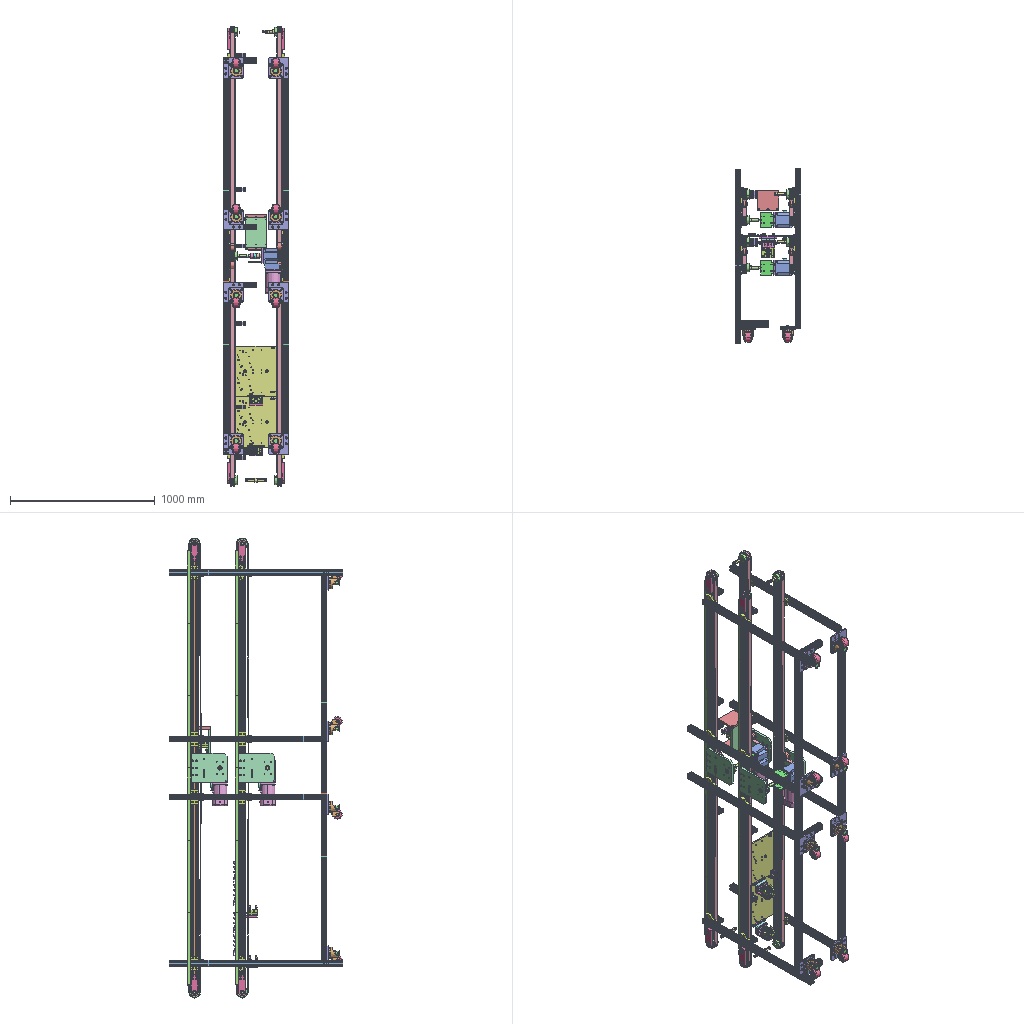Assembly | STEP file | 55 different items | 353 placed | box 456 x 1200 x 3179 mm
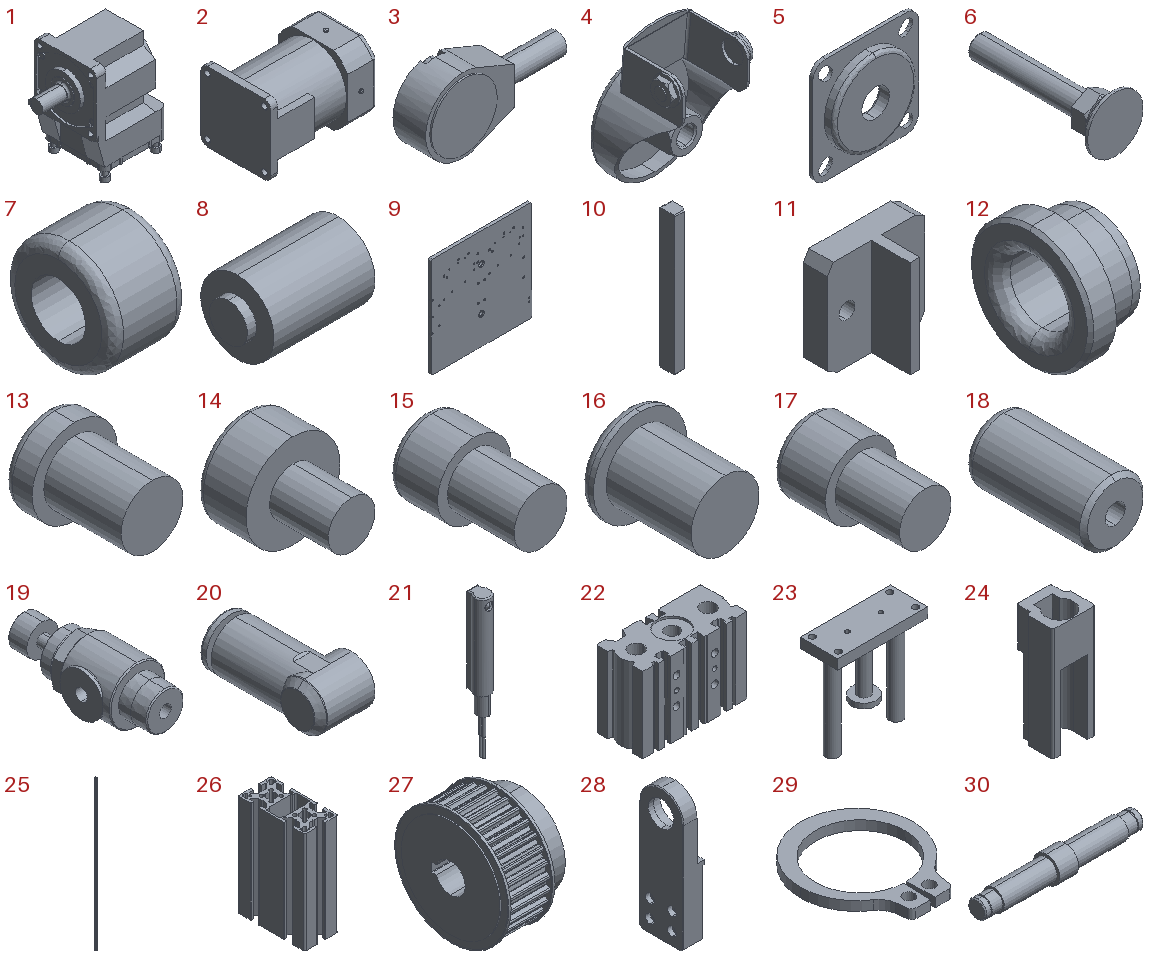Parts list (item | name | quantity | parent item | size | volume):
1 | - | x2 | in OM-BHI62E-5RA-CC05AC33P-EPCR1201-2_BHI62F_5RA_BH6G2_5RA05_, OM-BHI62E-5RA-CC05AC33P-EPCR1201-2_BHI62F_5RA_BH6G2_5RA05_-1 | 166 x 104 x 172.5 mm | 1495766 mm3
2 | OM-BHI62E-5RA-CC05AC33P-EPCR1201-2_200W_A_Motor-1 | x2 | in OM-BHI62E-5RA-CC05AC33P-EPCR1201-2_BHI62F_5RA_BH6G2_5RA05_, OM-BHI62E-5RA-CC05AC33P-EPCR1201-2_BHI62F_5RA_BH6G2_5RA05_-1 | 160 x 107.8 x 107.8 mm | 1356230 mm3
3 | OM-BHI62E-5RA-CC05AC33P-EPCR1201-2_Cable-1 | x2 | in OM-BHI62E-5RA-CC05AC33P-EPCR1201-2_BHI62F_5RA_BH6G2_5RA05_, OM-BHI62E-5RA-CC05AC33P-EPCR1201-2_BHI62F_5RA_BH6G2_5RA05_-1 | 53.5 x 14 x 27 mm | 9959 mm3
4 | CMA-2 | x8 | in CMAS65-F, CMAS65-F-1, CMAS65-F-2, CMAS65-F-3, CMAS65-F-4, CMAS65-F-5, CMAS65-F-6, CMAS65-F-7 | 80 x 61.3 x 107.359 mm | 51155 mm3
5 | CMA-1 | x8 | in CMAS65-F, CMAS65-F-1, CMAS65-F-2, CMAS65-F-3, CMAS65-F-4, CMAS65-F-5, CMAS65-F-6, CMAS65-F-7 | 102 x 12.8 x 102 mm | 66491 mm3
6 | CMA-5 | x8 | in CMAS65-F, CMAS65-F-1, CMAS65-F-2, CMAS65-F-3, CMAS65-F-4, CMAS65-F-5, CMAS65-F-6, CMAS65-F-7 | 40 x 98.8 x 40 mm | 27608 mm3
7 | CMA-4 | x8 | in CMAS65-F, CMAS65-F-1, CMAS65-F-2, CMAS65-F-3, CMAS65-F-4, CMAS65-F-5, CMAS65-F-6, CMAS65-F-7 | 45 x 65 x 65 mm | 108456 mm3
8 | CMA-3 | x8 | in CMAS65-F, CMAS65-F-1, CMAS65-F-2, CMAS65-F-3, CMAS65-F-4, CMAS65-F-5, CMAS65-F-6, CMAS65-F-7 | 53 x 32.5 x 32.5 mm | 39125 mm3
9 | PALL-001 | x2 | in PALL-01-ASSY, PALL-01-ASSY-1 | 350 x 10 x 348.5 mm | 1203530 mm3
10 | PALL-002 | x2 | in PALL-01-ASSY, PALL-01-ASSY-1 | 10 x 13 x 120 mm | 15010 mm3
11 | PALL-003 | x2 | in PALL-01-ASSY, PALL-01-ASSY-1 | 20 x 13 x 20 mm | 2211 mm3
12 | JBHM10-6 | x4 | in PALL-01-ASSY, PALL-01-ASSY-1 | 10 x 19 x 19 mm | 1348 mm3
13 | PALL-004 | x4 | in PALL-01-ASSY, PALL-01-ASSY-1 | 5.5 x 6.8 x 5.5 mm | 104.707 mm3
14 | PALL-005 | x8 | in PALL-01-ASSY, PALL-01-ASSY-1 | 8 x 9.13 x 8 mm | 269.118 mm3
15 | PALL-006 | x4 | in PALL-01-ASSY, PALL-01-ASSY-1 | 5.5 x 8.65 x 5.5 mm | 148.66 mm3
16 | PALL-007 | x8 | in PALL-01-ASSY, PALL-01-ASSY-1 | 5.5 x 5.8 x 5.5 mm | 80.949 mm3
17 | PALL-008 | x4 | in PALL-01-ASSY, PALL-01-ASSY-1 | 5.5 x 9.05 x 5.5 mm | 158.164 mm3
18 | PALL-009 | x44 | in PALL-01-ASSY, PALL-01-ASSY-1 | 8 x 15 x 8 mm | 707.835 mm3
19 | MGPL25-30-M9BL-U06US_AS3054 Body(23-01-06) | x6 | in MGPL25-30-M9BL-U06US_AS3054(AS2301F-01-06S), MGPL25-30-M9BL-U06US_AS3054(AS2301F-01-06S)-1, MGPL25-30-M9BL-U06US_AS3054(AS2301F-01-06S)-2, MGPL25-30-M9BL-U06US_AS3054(AS2301F-01-06S)-1-1, MGPL25-30-M9BL-U06US_AS3054(AS2301F-01-06S)-3, MGPL25-30-M9BL-U06US_AS3054(AS2301F-01-06S)-1-2 | 14.2 x 36.1 x 14.2 mm | 3404 mm3
20 | MGPL25-30-M9BL-U06US_AS3054 Uni Arm(2-01-06) | x6 | in MGPL25-30-M9BL-U06US_AS3054(AS2301F-01-06S), MGPL25-30-M9BL-U06US_AS3054(AS2301F-01-06S)-1, MGPL25-30-M9BL-U06US_AS3054(AS2301F-01-06S)-2, MGPL25-30-M9BL-U06US_AS3054(AS2301F-01-06S)-1-1, MGPL25-30-M9BL-U06US_AS3054(AS2301F-01-06S)-3, MGPL25-30-M9BL-U06US_AS3054(AS2301F-01-06S)-1-2 | 12.7 x 28.35 x 11.6 mm | 2524 mm3
21 | MGPL25-30-M9BL-U06US_F9_M9(M9B) | x6 | in MGPL25-30-M9BL-U06US_A9+F9+M9(M9B), MGPL25-30-M9BL-U06US_A9+F9+M9(M9B)-1, MGPL25-30-M9BL-U06US_A9+F9+M9(M9B)-2, MGPL25-30-M9BL-U06US_A9+F9+M9(M9B)-1-1, MGPL25-30-M9BL-U06US_A9+F9+M9(M9B)-3, MGPL25-30-M9BL-U06US_A9+F9+M9(M9B)-1-2 | 4 x 4.61 x 37 mm | 360.585 mm3
22 | MGPL25-30-M9BL-U06US_MGPTube(25L) | x3 | in MGPL25-30-M9BL-U06US(MGPL25-30-M9BL-U06US), MGPL25-30-M9BL-U06US(MGPL25-30-M9BL-U06US)-1, MGPL25-30-M9BL-U06US(MGPL25-30-M9BL-U06US-_flexible1) | 93 x 42 x 67.5 mm | 186060 mm3
23 | MGPL25-30-M9BL-U06US_MGPRod(25L) | x3 | in MGPL25-30-M9BL-U06US(MGPL25-30-M9BL-U06US), MGPL25-30-M9BL-U06US(MGPL25-30-M9BL-U06US)-1, MGPL25-30-M9BL-U06US(MGPL25-30-M9BL-U06US-_flexible1) | 91 x 38 x 99.5 mm | 65385 mm3
24 | MGPL25-30-M9BL-U06US_BMG2-012(Default) | x6 | in MGPL25-30-M9BL-U06US(MGPL25-30-M9BL-U06US), MGPL25-30-M9BL-U06US(MGPL25-30-M9BL-U06US)-1, MGPL25-30-M9BL-U06US(MGPL25-30-M9BL-U06US-_flexible1) | 6.2 x 5.9 x 16.5 mm | 235.85 mm3
25 | HFS5-2550-3000 | x4 | - | 25 x 50.001 x 3000 mm | 1510106 mm3
26 | HFS5-2550-300 | x11 | - | 25 x 50.001 x 76 mm | 38256 mm3
27 | HTPA30S8M250-B-N20-KC90-FC77.5-TPC5 | x12 | - | 48 x 77.5 x 77.5 mm | 160610 mm3
28 | CON-001 | x8 | - | 24 x 50 x 150 mm | 124182 mm3
29 | C Type Shaft Use Retaining Ring_jis(PreviewCfg) | x14 | - | 12.101 x 14.196 x 1 mm | 49.912 mm3
30 | CON-002 | x4 | - | 150 x 25 x 25 mm | 46152 mm3
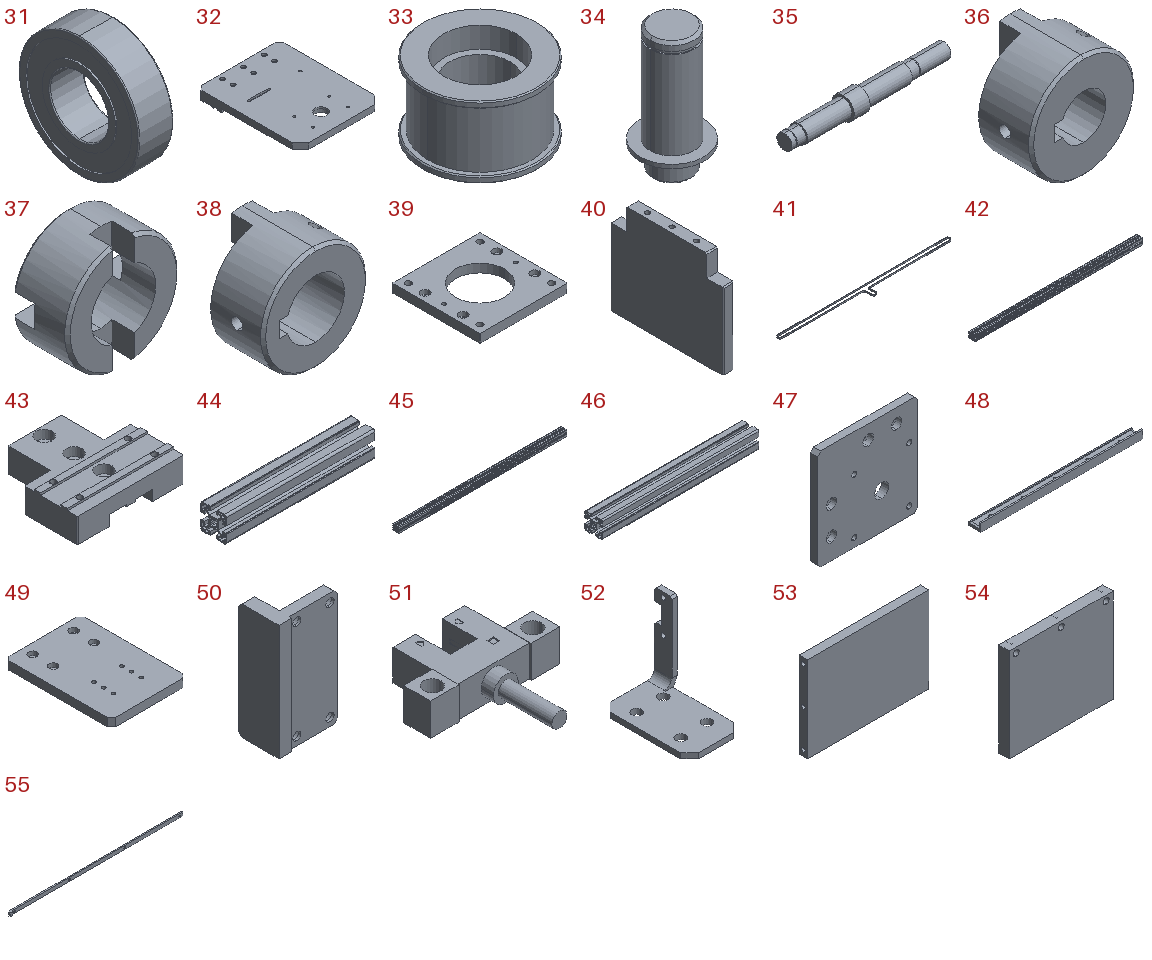31 | B6003ZZ | x25 | - | 10 x 35 x 35 mm | 7012 mm3
32 | CON-003 | x4 | - | 200 x 250 x 22 mm | 741218 mm3
33 | CON-004 | x8 | - | 55 x 55 x 34 mm | 40657 mm3
34 | CON-005 | x8 | - | 25 x 25 x 48.5 mm | 10531 mm3
35 | CON-006 | x2 | - | 180 x 25 x 25 mm | 52361 mm3
36 | CON-008 | x2 | - | 40 x 28 x 40 mm | 21406 mm3
37 | CON-009 | x2 | - | 40 x 20 x 40 mm | 14486 mm3
38 | CON-007 | x2 | - | 40 x 28 x 40 mm | 18074 mm3
39 | CON-010 | x2 | - | 104 x 104 x 10 mm | 77916 mm3
40 | CON-011 | x4 | - | 10 x 104 x 90 mm | 86051 mm3
41 | LTBR-S8M-840^ | x4 | - | 3180 x 255.872 x 25 mm | 890028 mm3
42 | AL PROFILE 4040 L 900 | x8 | - | 1050 x 40 x 40 mm | 583573 mm3
43 | CON-012 | x16 | - | 100 x 90 x 25 mm | 119624 mm3
44 | AL PROFILE 4040 L 456 | x4 | - | 233.35 x 40 x 40 mm | 129692 mm3
45 | AL PROFILE 4040 L 1110 | x4 | - | 1110 x 40 x 40 mm | 616920 mm3
46 | AL PROFILE 4040 L 360 | x2 | - | 360 x 40 x 40 mm | 200082 mm3
47 | CON-013 | x8 | - | 142 x 10 x 142 mm | 190361 mm3
48 | CON-016 | x24 | - | 500 x 37 x 24 mm | 214836 mm3
49 | CON-018 | x2 | - | 93 x 130 x 10 mm | 117582 mm3
50 | SCR-004 | x2 | - | 48 x 32 x 91 mm | 62029 mm3
51 | OMRON-EE_SX910P_R | x2 | - | 24 x 24.3 x 6 mm | 1063 mm3
52 | CON-019 | x2 | - | 33 x 50 x 47 mm | 5269 mm3
53 | CON-020 | x1 | - | 212 x 15 x 150 mm | 472548 mm3
54 | CON-021 | x2 | - | 150 x 15 x 135 mm | 298623 mm3
55 | CON-023 | x2 | - | 405 x 5 x 8 mm | 9596 mm3
Placements (level | parent | child | x y z in mm | rotation matrix by rows), first 336 of 380 lines:
1 | subassembly 2 | OM-BHI62E-5RA-CC05AC33P-EPCR1201-2_BHI62F_5RA_BH6G2_5RA05_ | 175.918 -181.25 23.458 | 0 0 -1 0 1 0 1 0 0
2 | OM-BHI62E-5RA-CC05AC33P-EPCR1201-2_BHI62F_5RA_BH6G2_5RA05_ | subassembly 3 | -0.0 -0.0 -0.0 | 0 0 1 0 1 0 -1 0 0
2 | OM-BHI62E-5RA-CC05AC33P-EPCR1201-2_BHI62F_5RA_BH6G2_5RA05_ | OM-BHI62E-5RA-CC05AC33P-EPCR1201-2_200W_A_Motor-1 | -112.0 0.0 -66.0 | -1 0 0 0 -1 0 0 0 1
2 | OM-BHI62E-5RA-CC05AC33P-EPCR1201-2_BHI62F_5RA_BH6G2_5RA05_ | OM-BHI62E-5RA-CC05AC33P-EPCR1201-2_Cable-1 | -116.2 52.0 -66.0 | -1 0 0 0 1 0 0 0 -1
1 | subassembly 2 | OM-BHI62E-5RA-CC05AC33P-EPCR1201-2_BHI62F_5RA_BH6G2_5RA05_-1 | 175.918 -511.25 23.458 | 0 0 -1 0 1 0 1 0 0
2 | OM-BHI62E-5RA-CC05AC33P-EPCR1201-2_BHI62F_5RA_BH6G2_5RA05_-1 | subassembly 3 | -0.0 -0.0 -0.0 | 0 0 1 0 1 0 -1 0 0
2 | OM-BHI62E-5RA-CC05AC33P-EPCR1201-2_BHI62F_5RA_BH6G2_5RA05_-1 | OM-BHI62E-5RA-CC05AC33P-EPCR1201-2_200W_A_Motor-1 | -112.0 0.0 -66.0 | -1 0 0 0 -1 0 0 0 1
2 | OM-BHI62E-5RA-CC05AC33P-EPCR1201-2_BHI62F_5RA_BH6G2_5RA05_-1 | OM-BHI62E-5RA-CC05AC33P-EPCR1201-2_Cable-1 | -116.2 52.0 -66.0 | -1 0 0 0 1 0 0 0 -1
1 | subassembly 2 | CMAS65-F | 261.918 -930.339 1302.458 | 1 0 0 0 1 0 0 0 1
2 | CMAS65-F | CMA-2 | -0.0 -0.0 -0.0 | 1 0 0 0 1 0 0 0 1
2 | CMAS65-F | CMA-1 | -0.0 -0.0 -0.0 | 1 0 0 0 1 0 0 0 1
2 | CMAS65-F | CMA-5 | -0.0 -0.0 -0.0 | 1 0 0 0 1 0 0 0 1
2 | CMAS65-F | CMA-4 | -0.0 -0.0 -0.0 | 1 0 0 0 1 0 0 0 1
2 | CMAS65-F | CMA-3 | -0.0 -0.0 -0.0 | 1 0 0 0 1 0 0 0 1
1 | subassembly 2 | CMAS65-F-1 | -12.082 -930.339 1302.458 | 1 0 0 0 1 0 0 0 1
2 | CMAS65-F-1 | CMA-2 | -0.0 -0.0 -0.0 | 1 0 0 0 1 0 0 0 1
2 | CMAS65-F-1 | CMA-1 | -0.0 -0.0 -0.0 | 1 0 0 0 1 0 0 0 1
2 | CMAS65-F-1 | CMA-5 | -0.0 -0.0 -0.0 | 1 0 0 0 1 0 0 0 1
2 | CMAS65-F-1 | CMA-4 | -0.0 -0.0 -0.0 | 1 0 0 0 1 0 0 0 1
2 | CMAS65-F-1 | CMA-3 | -0.0 -0.0 -0.0 | 1 0 0 0 1 0 0 0 1
1 | subassembly 2 | CMAS65-F-2 | 261.918 -930.339 -1255.542 | -1 0 0 0 1 0 0 0 -1
2 | CMAS65-F-2 | CMA-2 | -0.0 -0.0 -0.0 | 1 0 0 0 1 0 0 0 1
2 | CMAS65-F-2 | CMA-1 | -0.0 -0.0 -0.0 | 1 0 0 0 1 0 0 0 1
2 | CMAS65-F-2 | CMA-5 | -0.0 -0.0 -0.0 | 1 0 0 0 1 0 0 0 1
2 | CMAS65-F-2 | CMA-4 | -0.0 -0.0 -0.0 | 1 0 0 0 1 0 0 0 1
2 | CMAS65-F-2 | CMA-3 | -0.0 -0.0 -0.0 | 1 0 0 0 1 0 0 0 1
1 | subassembly 2 | CMAS65-F-3 | -12.082 -930.339 -1255.542 | -1 0 0 0 1 0 0 0 -1
2 | CMAS65-F-3 | CMA-2 | -0.0 -0.0 -0.0 | 1 0 0 0 1 0 0 0 1
2 | CMAS65-F-3 | CMA-1 | -0.0 -0.0 -0.0 | 1 0 0 0 1 0 0 0 1
2 | CMAS65-F-3 | CMA-5 | -0.0 -0.0 -0.0 | 1 0 0 0 1 0 0 0 1
2 | CMAS65-F-3 | CMA-4 | -0.0 -0.0 -0.0 | 1 0 0 0 1 0 0 0 1
2 | CMAS65-F-3 | CMA-3 | -0.0 -0.0 -0.0 | 1 0 0 0 1 0 0 0 1
1 | subassembly 2 | CMAS65-F-4 | 261.918 -930.339 294.458 | 1 0 0 0 1 0 0 0 1
2 | CMAS65-F-4 | CMA-2 | -0.0 -0.0 -0.0 | 1 0 0 0 1 0 0 0 1
2 | CMAS65-F-4 | CMA-1 | -0.0 -0.0 -0.0 | 1 0 0 0 1 0 0 0 1
2 | CMAS65-F-4 | CMA-5 | -0.0 -0.0 -0.0 | 1 0 0 0 1 0 0 0 1
2 | CMAS65-F-4 | CMA-4 | -0.0 -0.0 -0.0 | 1 0 0 0 1 0 0 0 1
2 | CMAS65-F-4 | CMA-3 | -0.0 -0.0 -0.0 | 1 0 0 0 1 0 0 0 1
1 | subassembly 2 | CMAS65-F-5 | -12.082 -930.339 294.458 | 1 0 0 0 1 0 0 0 1
2 | CMAS65-F-5 | CMA-2 | -0.0 -0.0 -0.0 | 1 0 0 0 1 0 0 0 1
2 | CMAS65-F-5 | CMA-1 | -0.0 -0.0 -0.0 | 1 0 0 0 1 0 0 0 1
2 | CMAS65-F-5 | CMA-5 | -0.0 -0.0 -0.0 | 1 0 0 0 1 0 0 0 1
2 | CMAS65-F-5 | CMA-4 | -0.0 -0.0 -0.0 | 1 0 0 0 1 0 0 0 1
2 | CMAS65-F-5 | CMA-3 | -0.0 -0.0 -0.0 | 1 0 0 0 1 0 0 0 1
1 | subassembly 2 | CMAS65-F-6 | 261.918 -930.339 -247.542 | -1 0 0 0 1 0 0 0 -1
2 | CMAS65-F-6 | CMA-2 | -0.0 -0.0 -0.0 | 1 0 0 0 1 0 0 0 1
2 | CMAS65-F-6 | CMA-1 | -0.0 -0.0 -0.0 | 1 0 0 0 1 0 0 0 1
2 | CMAS65-F-6 | CMA-5 | -0.0 -0.0 -0.0 | 1 0 0 0 1 0 0 0 1
2 | CMAS65-F-6 | CMA-4 | -0.0 -0.0 -0.0 | 1 0 0 0 1 0 0 0 1
2 | CMAS65-F-6 | CMA-3 | -0.0 -0.0 -0.0 | 1 0 0 0 1 0 0 0 1
1 | subassembly 2 | CMAS65-F-7 | -12.082 -930.339 -247.542 | -1 0 0 0 1 0 0 0 -1
2 | CMAS65-F-7 | CMA-2 | -0.0 -0.0 -0.0 | 1 0 0 0 1 0 0 0 1
2 | CMAS65-F-7 | CMA-1 | -0.0 -0.0 -0.0 | 1 0 0 0 1 0 0 0 1
2 | CMAS65-F-7 | CMA-5 | -0.0 -0.0 -0.0 | 1 0 0 0 1 0 0 0 1
2 | CMAS65-F-7 | CMA-4 | -0.0 -0.0 -0.0 | 1 0 0 0 1 0 0 0 1
2 | CMAS65-F-7 | CMA-3 | -0.0 -0.0 -0.0 | 1 0 0 0 1 0 0 0 1
1 | subassembly 2 | PALL-01-ASSY | 142.834 -295.188 -1083.871 | 0 0 -1 0 1 0 1 0 -0
2 | PALL-01-ASSY | PALL-001 | -40.171 -0.1701 17.916 | 1 0 0 0 1 0 0 0 1
2 | PALL-01-ASSY | PALL-002 | -210.171 -13.17 17.916 | 1 0 0 0 1 0 0 0 1
2 | PALL-01-ASSY | PALL-003 | 124.829 -13.17 -97.084 | 0 0 -1 0 1 0 1 0 -0
2 | PALL-01-ASSY | JBHM10-6 | -40.171 -0.6701 92.916 | 0 -1 0 1 0 0 0 0 1
2 | PALL-01-ASSY | JBHM10-6 | -40.171 -0.6701 -57.084 | 0 -1 0 1 0 0 0 0 1
2 | PALL-01-ASSY | PALL-004 | 5.829 4.83 132.516 | 1 0 0 0 1 0 0 0 1
2 | PALL-01-ASSY | PALL-004 | -151.671 4.83 132.516 | -0.04381 0 0.999 0 1 0 -0.999 0 -0.04381
2 | PALL-01-ASSY | PALL-005 | 15.929 4.83 60.546 | 1 0 0 0 1 0 0 0 1
2 | PALL-01-ASSY | PALL-005 | 91.249 4.83 88.726 | 1 0 0 0 1 0 0 0 1
2 | PALL-01-ASSY | PALL-005 | -141.571 4.83 60.546 | 1 0 0 0 1 0 0 0 1
2 | PALL-01-ASSY | PALL-005 | -66.251 4.83 88.726 | 1 0 0 0 1 0 0 0 1
2 | PALL-01-ASSY | PALL-006 | -120.871 4.83 136.246 | 0.9997 0 -0.02348 0 1 0 0.02348 0 0.9997
2 | PALL-01-ASSY | PALL-006 | 36.699 4.83 136.246 | -0.5733 0 0.8194 0 1 0 -0.8194 0 -0.5733
2 | PALL-01-ASSY | PALL-007 | -64.941 4.83 106.708 | 1 0 0 0 1 0 0 0 1
2 | PALL-01-ASSY | PALL-007 | 60.357 4.83 138.448 | 1 0 0 0 1 0 0 0 1
2 | PALL-01-ASSY | PALL-007 | 92.559 4.83 106.708 | 1 0 0 0 1 0 0 0 1
2 | PALL-01-ASSY | PALL-007 | -97.143 4.83 138.448 | 1 0 0 0 1 0 0 0 1
2 | PALL-01-ASSY | PALL-008 | 61.281 4.83 68.085 | 1 0 0 0 1 0 0 0 1
2 | PALL-01-ASSY | PALL-008 | -96.219 4.83 68.085 | 1 0 0 0 1 0 0 0 1
2 | PALL-01-ASSY | PALL-009 | 106.629 4.83 39.966 | 1 0 0 0 1 0 0 0 1
2 | PALL-01-ASSY | PALL-009 | 104.329 4.83 129.966 | 1 0 0 0 1 0 0 0 1
2 | PALL-01-ASSY | PALL-009 | -2.171 4.83 111.966 | 0.6681 0 -0.7441 0 1 0 0.7441 0 0.6681
2 | PALL-01-ASSY | PALL-009 | -85.871 4.83 146.166 | 1 0 0 0 1 0 0 0 1
2 | PALL-01-ASSY | PALL-009 | 106.629 4.83 -20.034 | 1 0 0 0 1 0 0 0 1
2 | PALL-01-ASSY | PALL-009 | -29.371 4.83 39.966 | 1 0 0 0 1 0 0 0 1
2 | PALL-01-ASSY | PALL-009 | -159.671 4.83 111.966 | 0.6681 0 -0.7441 0 1 0 0.7441 0 0.6681
2 | PALL-01-ASSY | PALL-009 | -170.071 4.83 49.966 | 1 0 0 0 1 0 0 0 1
2 | PALL-01-ASSY | PALL-009 | -12.571 4.83 49.966 | 1 0 0 0 1 0 0 0 1
2 | PALL-01-ASSY | PALL-009 | 71.629 4.83 146.166 | 1 0 0 0 1 0 0 0 1
2 | PALL-01-ASSY | PALL-009 | -50.871 4.83 39.966 | 1 0 0 0 1 0 0 0 1
2 | PALL-01-ASSY | PALL-009 | -170.071 4.83 121.266 | 1 0 0 0 1 0 0 0 1
2 | PALL-01-ASSY | PALL-009 | -118.871 4.83 146.166 | 1 0 0 0 1 0 0 0 1
2 | PALL-01-ASSY | PALL-009 | -53.171 4.83 129.966 | 1 0 0 0 1 0 0 0 1
2 | PALL-01-ASSY | PALL-009 | -12.571 4.83 121.266 | 1 0 0 0 1 0 0 0 1
2 | PALL-01-ASSY | PALL-009 | -29.371 4.83 -20.034 | 1 0 0 0 1 0 0 0 1
2 | PALL-01-ASSY | PALL-009 | -50.871 4.83 -20.034 | 1 0 0 0 1 0 0 0 1
2 | PALL-01-ASSY | PALL-009 | -186.871 4.83 39.966 | 1 0 0 0 1 0 0 0 1
2 | PALL-01-ASSY | PALL-009 | -186.871 4.83 -20.034 | 1 0 0 0 1 0 0 0 1
2 | PALL-01-ASSY | PALL-009 | 104.329 4.83 104.966 | 1 0 0 0 1 0 0 0 1
2 | PALL-01-ASSY | PALL-009 | -53.171 4.83 104.966 | 1 0 0 0 1 0 0 0 1
2 | PALL-01-ASSY | PALL-009 | 38.629 4.83 146.166 | 1 0 0 0 1 0 0 0 1
1 | subassembly 2 | PALL-01-ASSY-1 | 142.834 -295.188 -733.871 | 0 0 -1 0 1 0 1 0 -0
2 | PALL-01-ASSY-1 | PALL-001 | -40.171 -0.1701 17.916 | 1 0 0 0 1 0 0 0 1
2 | PALL-01-ASSY-1 | PALL-002 | -210.171 -13.17 17.916 | 1 0 0 0 1 0 0 0 1
2 | PALL-01-ASSY-1 | PALL-003 | 124.829 -13.17 -97.084 | 0 0 -1 0 1 0 1 0 -0
2 | PALL-01-ASSY-1 | JBHM10-6 | -40.171 -0.6701 92.916 | 0 -1 0 1 0 0 0 0 1
2 | PALL-01-ASSY-1 | JBHM10-6 | -40.171 -0.6701 -57.084 | 0 -1 0 1 0 0 0 0 1
2 | PALL-01-ASSY-1 | PALL-004 | 5.829 4.83 132.516 | 1 0 0 0 1 0 0 0 1
2 | PALL-01-ASSY-1 | PALL-004 | -151.671 4.83 132.516 | -0.04381 0 0.999 0 1 0 -0.999 0 -0.04381
2 | PALL-01-ASSY-1 | PALL-005 | 15.929 4.83 60.546 | 1 0 0 0 1 0 0 0 1
2 | PALL-01-ASSY-1 | PALL-005 | -66.251 4.83 88.726 | 1 0 0 0 1 0 0 0 1
2 | PALL-01-ASSY-1 | PALL-005 | -141.571 4.83 60.546 | 1 0 0 0 1 0 0 0 1
2 | PALL-01-ASSY-1 | PALL-005 | 91.249 4.83 88.726 | 1 0 0 0 1 0 0 0 1
2 | PALL-01-ASSY-1 | PALL-006 | 36.699 4.83 136.246 | -0.5733 0 0.8194 0 1 0 -0.8194 0 -0.5733
2 | PALL-01-ASSY-1 | PALL-006 | -120.871 4.83 136.246 | 0.9997 0 -0.02348 0 1 0 0.02348 0 0.9997
2 | PALL-01-ASSY-1 | PALL-007 | 92.559 4.83 106.708 | 1 0 0 0 1 0 0 0 1
2 | PALL-01-ASSY-1 | PALL-007 | 60.357 4.83 138.448 | 1 0 0 0 1 0 0 0 1
2 | PALL-01-ASSY-1 | PALL-007 | -97.143 4.83 138.448 | 1 0 0 0 1 0 0 0 1
2 | PALL-01-ASSY-1 | PALL-007 | -64.941 4.83 106.708 | 1 0 0 0 1 0 0 0 1
2 | PALL-01-ASSY-1 | PALL-008 | 61.281 4.83 68.085 | 1 0 0 0 1 0 0 0 1
2 | PALL-01-ASSY-1 | PALL-008 | -96.219 4.83 68.085 | 1 0 0 0 1 0 0 0 1
2 | PALL-01-ASSY-1 | PALL-009 | -2.171 4.83 111.966 | 0.6681 0 -0.7441 0 1 0 0.7441 0 0.6681
2 | PALL-01-ASSY-1 | PALL-009 | -170.071 4.83 121.266 | 1 0 0 0 1 0 0 0 1
2 | PALL-01-ASSY-1 | PALL-009 | -12.571 4.83 121.266 | 1 0 0 0 1 0 0 0 1
2 | PALL-01-ASSY-1 | PALL-009 | -118.871 4.83 146.166 | 1 0 0 0 1 0 0 0 1
2 | PALL-01-ASSY-1 | PALL-009 | -29.371 4.83 39.966 | 1 0 0 0 1 0 0 0 1
2 | PALL-01-ASSY-1 | PALL-009 | -85.871 4.83 146.166 | 1 0 0 0 1 0 0 0 1
2 | PALL-01-ASSY-1 | PALL-009 | -159.671 4.83 111.966 | 0.6681 0 -0.7441 0 1 0 0.7441 0 0.6681
2 | PALL-01-ASSY-1 | PALL-009 | 104.329 4.83 129.966 | 1 0 0 0 1 0 0 0 1
2 | PALL-01-ASSY-1 | PALL-009 | 104.329 4.83 104.966 | 1 0 0 0 1 0 0 0 1
2 | PALL-01-ASSY-1 | PALL-009 | 71.629 4.83 146.166 | 1 0 0 0 1 0 0 0 1
2 | PALL-01-ASSY-1 | PALL-009 | 38.629 4.83 146.166 | 1 0 0 0 1 0 0 0 1
2 | PALL-01-ASSY-1 | PALL-009 | -186.871 4.83 39.966 | 1 0 0 0 1 0 0 0 1
2 | PALL-01-ASSY-1 | PALL-009 | -186.871 4.83 -20.034 | 1 0 0 0 1 0 0 0 1
2 | PALL-01-ASSY-1 | PALL-009 | -170.071 4.83 49.966 | 1 0 0 0 1 0 0 0 1
2 | PALL-01-ASSY-1 | PALL-009 | 106.629 4.83 39.966 | 1 0 0 0 1 0 0 0 1
2 | PALL-01-ASSY-1 | PALL-009 | 106.629 4.83 -20.034 | 1 0 0 0 1 0 0 0 1
2 | PALL-01-ASSY-1 | PALL-009 | -29.371 4.83 -20.034 | 1 0 0 0 1 0 0 0 1
2 | PALL-01-ASSY-1 | PALL-009 | -50.871 4.83 -20.034 | 1 0 0 0 1 0 0 0 1
2 | PALL-01-ASSY-1 | PALL-009 | -12.571 4.83 49.966 | 1 0 0 0 1 0 0 0 1
2 | PALL-01-ASSY-1 | PALL-009 | -53.171 4.83 104.966 | 1 0 0 0 1 0 0 0 1
2 | PALL-01-ASSY-1 | PALL-009 | -53.171 4.83 129.966 | 1 0 0 0 1 0 0 0 1
2 | PALL-01-ASSY-1 | PALL-009 | -50.871 4.83 39.966 | 1 0 0 0 1 0 0 0 1
1 | subassembly 2 | MGPL25-30-M9BL-U06US(MGPL25-30-M9BL-U06US) | 124.918 -406.589 -1328.042 | -1 0 0 0 0 1 0 1 0
2 | MGPL25-30-M9BL-U06US(MGPL25-30-M9BL-U06US) | MGPL25-30-M9BL-U06US_AS3054(AS2301F-01-06S) | 28.5 31.3 -24.75 | -1 0 0 0 1 0 0 0 -1
3 | MGPL25-30-M9BL-U06US_AS3054(AS2301F-01-06S) | MGPL25-30-M9BL-U06US_AS3054 Body(23-01-06) | -0.0 0.0 -0.0 | 1 0 0 0 1 0 0 0 1
3 | MGPL25-30-M9BL-U06US_AS3054(AS2301F-01-06S) | MGPL25-30-M9BL-U06US_AS3054 Uni Arm(2-01-06) | -7.1 -0.0 -0.0 | 1 0 0 0 1 0 0 0 1
2 | MGPL25-30-M9BL-U06US(MGPL25-30-M9BL-U06US) | MGPL25-30-M9BL-U06US_AS3054(AS2301F-01-06S)-1 | 28.5 31.3 22.25 | -1 0 0 0 1 0 0 0 -1
3 | MGPL25-30-M9BL-U06US_AS3054(AS2301F-01-06S)-1 | MGPL25-30-M9BL-U06US_AS3054 Body(23-01-06) | -0.0 -0.0 -0.0 | 1 0 0 0 1 0 0 0 1
3 | MGPL25-30-M9BL-U06US_AS3054(AS2301F-01-06S)-1 | MGPL25-30-M9BL-U06US_AS3054 Uni Arm(2-01-06) | -7.1 0.0 -0.0 | 1 0 0 0 1 0 0 0 1
2 | MGPL25-30-M9BL-U06US(MGPL25-30-M9BL-U06US) | MGPL25-30-M9BL-U06US_A9+F9+M9(M9B) | 5.5 16.311 29.25 | 1 0 0 0 1 0 0 0 1
3 | MGPL25-30-M9BL-U06US_A9+F9+M9(M9B) | MGPL25-30-M9BL-U06US_F9_M9(M9B) | -0.0 -0.0 -0.0 | 1 0 0 0 1 0 0 0 1
2 | MGPL25-30-M9BL-U06US(MGPL25-30-M9BL-U06US) | MGPL25-30-M9BL-U06US_A9+F9+M9(M9B)-1 | -5.5 16.311 -25.75 | -1 0 0 0 1 0 0 0 -1
3 | MGPL25-30-M9BL-U06US_A9+F9+M9(M9B)-1 | MGPL25-30-M9BL-U06US_F9_M9(M9B) | -0.0 0.0 0.0 | 1 0 0 0 1 0 0 0 1
2 | MGPL25-30-M9BL-U06US(MGPL25-30-M9BL-U06US) | MGPL25-30-M9BL-U06US_MGPTube(25L) | -0.0 -0.0 -0.0 | 1 0 0 0 1 0 0 0 1
2 | MGPL25-30-M9BL-U06US(MGPL25-30-M9BL-U06US) | MGPL25-30-M9BL-U06US_MGPRod(25L) | -0.0 -0.0 15.0 | 1 0 0 0 1 0 0 0 1
2 | MGPL25-30-M9BL-U06US(MGPL25-30-M9BL-U06US) | MGPL25-30-M9BL-U06US_BMG2-012(Default) | 5.5 16.311 21.0 | 1 0 0 0 1 0 0 0 1
2 | MGPL25-30-M9BL-U06US(MGPL25-30-M9BL-U06US) | MGPL25-30-M9BL-U06US_BMG2-012(Default) | -5.5 16.311 -17.5 | -1 0 0 0 1 0 0 0 -1
1 | subassembly 2 | MGPL25-30-M9BL-U06US(MGPL25-30-M9BL-U06US)-1 | 124.918 -406.589 -978.042 | -1 0 0 0 0 1 0 1 0
2 | MGPL25-30-M9BL-U06US(MGPL25-30-M9BL-U06US)-1 | MGPL25-30-M9BL-U06US_AS3054(AS2301F-01-06S)-2 | 28.5 31.3 -24.75 | -1 0 0 0 1 0 0 0 -1
3 | MGPL25-30-M9BL-U06US_AS3054(AS2301F-01-06S)-2 | MGPL25-30-M9BL-U06US_AS3054 Body(23-01-06) | -0.0 0.0 -0.0 | 1 0 0 0 1 0 0 0 1
3 | MGPL25-30-M9BL-U06US_AS3054(AS2301F-01-06S)-2 | MGPL25-30-M9BL-U06US_AS3054 Uni Arm(2-01-06) | -7.1 -0.0 -0.0 | 1 0 0 0 1 0 0 0 1
2 | MGPL25-30-M9BL-U06US(MGPL25-30-M9BL-U06US)-1 | MGPL25-30-M9BL-U06US_AS3054(AS2301F-01-06S)-1-1 | 28.5 31.3 22.25 | -1 0 0 0 1 0 0 0 -1
3 | MGPL25-30-M9BL-U06US_AS3054(AS2301F-01-06S)-1-1 | MGPL25-30-M9BL-U06US_AS3054 Body(23-01-06) | -0.0 -0.0 -0.0 | 1 0 0 0 1 0 0 0 1
3 | MGPL25-30-M9BL-U06US_AS3054(AS2301F-01-06S)-1-1 | MGPL25-30-M9BL-U06US_AS3054 Uni Arm(2-01-06) | -7.1 0.0 -0.0 | 1 0 0 0 1 0 0 0 1
2 | MGPL25-30-M9BL-U06US(MGPL25-30-M9BL-U06US)-1 | MGPL25-30-M9BL-U06US_A9+F9+M9(M9B)-2 | 5.5 16.311 29.25 | 1 0 0 0 1 0 0 0 1
3 | MGPL25-30-M9BL-U06US_A9+F9+M9(M9B)-2 | MGPL25-30-M9BL-U06US_F9_M9(M9B) | -0.0 -0.0 -0.0 | 1 0 0 0 1 0 0 0 1
2 | MGPL25-30-M9BL-U06US(MGPL25-30-M9BL-U06US)-1 | MGPL25-30-M9BL-U06US_A9+F9+M9(M9B)-1-1 | -5.5 16.311 -25.75 | -1 0 0 0 1 0 0 0 -1
3 | MGPL25-30-M9BL-U06US_A9+F9+M9(M9B)-1-1 | MGPL25-30-M9BL-U06US_F9_M9(M9B) | -0.0 0.0 0.0 | 1 0 0 0 1 0 0 0 1
2 | MGPL25-30-M9BL-U06US(MGPL25-30-M9BL-U06US)-1 | MGPL25-30-M9BL-U06US_MGPTube(25L) | -0.0 -0.0 -0.0 | 1 0 0 0 1 0 0 0 1
2 | MGPL25-30-M9BL-U06US(MGPL25-30-M9BL-U06US)-1 | MGPL25-30-M9BL-U06US_MGPRod(25L) | -0.0 -0.0 15.0 | 1 0 0 0 1 0 0 0 1
2 | MGPL25-30-M9BL-U06US(MGPL25-30-M9BL-U06US)-1 | MGPL25-30-M9BL-U06US_BMG2-012(Default) | 5.5 16.311 21.0 | 1 0 0 0 1 0 0 0 1
2 | MGPL25-30-M9BL-U06US(MGPL25-30-M9BL-U06US)-1 | MGPL25-30-M9BL-U06US_BMG2-012(Default) | -5.5 16.311 -17.5 | -1 0 0 0 1 0 0 0 -1
1 | subassembly 2 | MGPL25-30-M9BL-U06US(MGPL25-30-M9BL-U06US-_flexible1) | 124.918 -66.589 186.458 | 1 0 0 0 0 1 0 -1 0
2 | MGPL25-30-M9BL-U06US(MGPL25-30-M9BL-U06US-_flexible1) | MGPL25-30-M9BL-U06US_AS3054(AS2301F-01-06S)-3 | 28.5 31.3 -24.75 | -1 0 0 0 1 0 0 0 -1
3 | MGPL25-30-M9BL-U06US_AS3054(AS2301F-01-06S)-3 | MGPL25-30-M9BL-U06US_AS3054 Body(23-01-06) | -0.0 -0.0 -0.0 | 1 0 0 0 1 0 0 0 1
3 | MGPL25-30-M9BL-U06US_AS3054(AS2301F-01-06S)-3 | MGPL25-30-M9BL-U06US_AS3054 Uni Arm(2-01-06) | -7.1 0.0 -0.0 | 1 0 0 0 1 0 0 0 1
2 | MGPL25-30-M9BL-U06US(MGPL25-30-M9BL-U06US-_flexible1) | MGPL25-30-M9BL-U06US_AS3054(AS2301F-01-06S)-1-2 | 28.5 31.3 22.25 | -1 0 0 0 1 0 0 0 -1
3 | MGPL25-30-M9BL-U06US_AS3054(AS2301F-01-06S)-1-2 | MGPL25-30-M9BL-U06US_AS3054 Body(23-01-06) | -0.0 -0.0 -0.0 | 1 0 0 0 1 0 0 0 1
3 | MGPL25-30-M9BL-U06US_AS3054(AS2301F-01-06S)-1-2 | MGPL25-30-M9BL-U06US_AS3054 Uni Arm(2-01-06) | -7.1 0.0 -0.0 | 1 0 0 0 1 0 0 0 1
2 | MGPL25-30-M9BL-U06US(MGPL25-30-M9BL-U06US-_flexible1) | MGPL25-30-M9BL-U06US_A9+F9+M9(M9B)-3 | 5.5 16.311 29.25 | 1 0 0 0 1 0 0 0 1
3 | MGPL25-30-M9BL-U06US_A9+F9+M9(M9B)-3 | MGPL25-30-M9BL-U06US_F9_M9(M9B) | -0.0 -0.0 -0.0 | 1 0 0 0 1 0 0 0 1
2 | MGPL25-30-M9BL-U06US(MGPL25-30-M9BL-U06US-_flexible1) | MGPL25-30-M9BL-U06US_A9+F9+M9(M9B)-1-2 | -5.5 16.311 -25.75 | -1 0 0 0 1 0 0 0 -1
3 | MGPL25-30-M9BL-U06US_A9+F9+M9(M9B)-1-2 | MGPL25-30-M9BL-U06US_F9_M9(M9B) | -0.0 -0.0 -0.0 | 1 0 0 0 1 0 0 0 1
2 | MGPL25-30-M9BL-U06US(MGPL25-30-M9BL-U06US-_flexible1) | MGPL25-30-M9BL-U06US_MGPTube(25L) | -0.0 -0.0 -0.0 | 1 0 0 0 1 0 0 0 1
2 | MGPL25-30-M9BL-U06US(MGPL25-30-M9BL-U06US-_flexible1) | MGPL25-30-M9BL-U06US_MGPRod(25L) | 0.0 0.0 15.0 | 1 0 0 0 1 0 0 0 1
2 | MGPL25-30-M9BL-U06US(MGPL25-30-M9BL-U06US-_flexible1) | MGPL25-30-M9BL-U06US_BMG2-012(Default) | -5.5 16.311 -17.5 | -1 0 0 0 1 0 0 0 -1
2 | MGPL25-30-M9BL-U06US(MGPL25-30-M9BL-U06US-_flexible1) | MGPL25-30-M9BL-U06US_BMG2-012(Default) | 5.5 16.311 21.0 | 1 0 0 0 1 0 0 0 1
1 | subassembly 2 | HFS5-2550-3000 | 287.418 -5.339 1523.458 | 1 0 0 0 1 0 0 0 1
1 | subassembly 2 | HFS5-2550-3000 | 287.418 -335.339 1523.458 | 1 0 0 0 1 0 0 0 1
1 | subassembly 2 | HFS5-2550-3000 | -37.582 -335.339 1523.458 | 1 0 0 0 1 0 0 0 1
1 | subassembly 2 | HFS5-2550-3000 | -37.582 -5.339 1523.458 | 1 0 0 0 1 0 0 0 1
1 | subassembly 2 | HFS5-2550-300 | -25.082 -335.339 -1371.542 | 0 0 -1 0 1 0 1 0 -0
1 | subassembly 2 | HFS5-2550-300 | -25.082 -5.339 92.958 | 0 0 -1 0 1 0 1 0 0
1 | subassembly 2 | HFS5-2550-300 | -25.082 -5.339 -1371.542 | 0 0 -1 0 1 0 1 0 -0
1 | subassembly 2 | HFS5-2550-300 | -25.082 -335.339 483.458 | 0 0 -1 0 1 0 1 0 -0
1 | subassembly 2 | HFS5-2550-300 | -25.082 -5.339 483.458 | 0 0 -1 0 1 0 1 0 -0
1 | subassembly 2 | HFS5-2550-300 | -25.082 -335.339 -1021.542 | 0 0 -1 0 1 0 1 0 0
1 | subassembly 2 | HFS5-2550-300 | -25.082 -335.339 -444.042 | 0 0 -1 0 1 0 1 0 -0
1 | subassembly 2 | HFS5-2550-300 | -25.082 -5.339 -444.042 | 0 0 -1 0 1 0 1 0 -0
1 | subassembly 2 | HFS5-2550-300 | -25.082 -5.339 279.958 | 0 0 -1 0 1 0 1 0 0
1 | subassembly 2 | HFS5-2550-300 | -25.082 -5.339 1410.958 | 0 0 -1 0 1 0 1 0 -0
1 | subassembly 2 | HFS5-2550-300 | -25.082 -335.339 1410.958 | 0 0 -1 0 1 0 1 0 -0
1 | subassembly 2 | HTPA30S8M250-B-N20-KC90-FC77.5-TPC5 | 303.918 -5.339 1573.458 | -1 0 0 0 -0.959 -0.2833 0 -0.2833 0.959
1 | subassembly 2 | HTPA30S8M250-B-N20-KC90-FC77.5-TPC5 | 303.918 -5.339 -1526.542 | -1 0 0 0 0.7382 0.6746 0 0.6746 -0.7382
1 | subassembly 2 | HTPA30S8M250-B-N20-KC90-FC77.5-TPC5 | 303.918 -181.25 23.458 | -1 0 0 0 0.5005 -0.8657 0 -0.8657 -0.5005
1 | subassembly 2 | HTPA30S8M250-B-N20-KC90-FC77.5-TPC5 | -54.082 -335.339 1573.458 | 1 0 0 0 -0.959 0.2833 0 -0.2833 -0.959
1 | subassembly 2 | HTPA30S8M250-B-N20-KC90-FC77.5-TPC5 | -54.082 -5.339 -1526.542 | 1 0 0 0 0.7382 -0.6746 0 0.6746 0.7382
1 | subassembly 2 | HTPA30S8M250-B-N20-KC90-FC77.5-TPC5 | 303.918 -511.25 23.458 | -1 0 0 0 0.5005 -0.8657 0 -0.8657 -0.5005
1 | subassembly 2 | HTPA30S8M250-B-N20-KC90-FC77.5-TPC5 | 303.918 -335.339 -1526.542 | -1 0 0 0 0.7382 0.6746 0 0.6746 -0.7382
1 | subassembly 2 | HTPA30S8M250-B-N20-KC90-FC77.5-TPC5 | -54.082 -511.25 23.458 | 1 0 0 0 0.5005 0.8657 0 -0.8657 0.5005
1 | subassembly 2 | HTPA30S8M250-B-N20-KC90-FC77.5-TPC5 | 303.918 -335.339 1573.458 | -1 0 0 0 -0.959 -0.2833 0 -0.2833 0.959
1 | subassembly 2 | HTPA30S8M250-B-N20-KC90-FC77.5-TPC5 | -54.082 -5.339 1573.458 | 1 0 0 0 -0.959 0.2833 0 -0.2833 -0.959
1 | subassembly 2 | HTPA30S8M250-B-N20-KC90-FC77.5-TPC5 | -54.082 -181.25 23.458 | 1 0 0 0 0.5005 0.8657 0 -0.8657 0.5005
1 | subassembly 2 | HTPA30S8M250-B-N20-KC90-FC77.5-TPC5 | -54.082 -335.339 -1526.542 | 1 0 0 0 0.7382 -0.6746 0 0.6746 0.7382
1 | subassembly 2 | CON-001 | -72.082 -335.339 1573.458 | 1 0 0 0 1 0 0 0 1
1 | subassembly 2 | CON-001 | -72.082 -335.339 -1526.542 | 1 0 0 0 -1 0 0 0 -1
1 | subassembly 2 | CON-001 | 321.918 -5.339 -1526.542 | -1 0 0 0 1 0 0 0 -1
1 | subassembly 2 | CON-001 | 321.918 -335.339 -1526.542 | -1 0 0 0 1 0 0 0 -1
1 | subassembly 2 | CON-001 | -72.082 -5.339 1573.458 | 1 0 0 0 1 0 0 0 1
1 | subassembly 2 | CON-001 | 321.918 -335.339 1573.458 | -1 0 0 0 -1 0 0 0 1
1 | subassembly 2 | CON-001 | -72.082 -5.339 -1526.542 | 1 0 0 0 -1 0 0 0 -1
1 | subassembly 2 | CON-001 | 321.918 -5.339 1573.458 | -1 0 0 0 -1 0 0 0 1
1 | subassembly 2 | C Type Shaft Use Retaining Ring_jis(PreviewCfg) | 177.918 -5.339 1573.458 | 0 0 1 0 1 0 -1 0 -0
1 | subassembly 2 | C Type Shaft Use Retaining Ring_jis(PreviewCfg) | 316.918 -335.339 -1526.542 | 0 0 1 -0.966 0.2586 0 -0.2586 -0.966 -0
1 | subassembly 2 | C Type Shaft Use Retaining Ring_jis(PreviewCfg) | -67.082 -180.339 23.458 | 0 0 -1 0 1 0 1 0 0
1 | subassembly 2 | C Type Shaft Use Retaining Ring_jis(PreviewCfg) | 55.918 -335.339 -1526.542 | 0 0 1 0 1 0 -1 0 -0
1 | subassembly 2 | C Type Shaft Use Retaining Ring_jis(PreviewCfg) | 177.918 -335.339 1573.458 | 0 0 1 0 1 0 -1 0 -0
1 | subassembly 2 | C Type Shaft Use Retaining Ring_jis(PreviewCfg) | 193.918 -335.339 -1526.542 | 0 0 -1 0 1 0 1 0 0
1 | subassembly 2 | C Type Shaft Use Retaining Ring_jis(PreviewCfg) | 10.447 -11.922 1567.084 | 0 0 -1 0 1 0 1 0 -0
1 | subassembly 2 | C Type Shaft Use Retaining Ring_jis(PreviewCfg) | 316.918 -5.339 -1526.542 | 0 0 1 -0.966 0.2586 0 -0.2586 -0.966 -0
1 | subassembly 2 | C Type Shaft Use Retaining Ring_jis(PreviewCfg) | 315.918 -335.339 1573.458 | 0 0 -1 0 1 0 1 0 0
1 | subassembly 2 | C Type Shaft Use Retaining Ring_jis(PreviewCfg) | 55.918 -5.339 -1526.542 | 0 0 1 0 1 0 -1 0 -0
1 | subassembly 2 | C Type Shaft Use Retaining Ring_jis(PreviewCfg) | 249.547 -6.169 1571.864 | 0 0 1 0 1 0 -1 0 -0
1 | subassembly 2 | C Type Shaft Use Retaining Ring_jis(PreviewCfg) | 315.918 -5.339 1573.458 | 0 0 -1 0 1 0 1 0 0
1 | subassembly 2 | C Type Shaft Use Retaining Ring_jis(PreviewCfg) | 193.918 -5.339 -1526.542 | 0 0 -1 0 1 0 1 0 0
1 | subassembly 2 | C Type Shaft Use Retaining Ring_jis(PreviewCfg) | 316.918 -180.339 23.458 | 0 0 1 0 1 0 -1 0 0
1 | subassembly 2 | CON-002 | 124.918 -5.339 -1526.542 | 1 0 0 0 0.7382 -0.6746 0 0.6746 0.7382
1 | subassembly 2 | CON-002 | 246.918 -335.339 1573.458 | 1 0 0 0 -0.959 0.2833 0 -0.2833 -0.959
1 | subassembly 2 | CON-002 | 246.918 -5.339 1573.458 | 1 0 0 0 -0.959 0.2833 0 -0.2833 -0.959
1 | subassembly 2 | CON-002 | 124.918 -335.339 -1526.542 | 1 0 0 0 0.7382 -0.6746 0 0.6746 0.7382
1 | subassembly 2 | B6003ZZ | -30.582 -401.25 -41.542 | 1 0 0 0 1 0 0 0 1
1 | subassembly 2 | B6003ZZ | 294.418 -71.25 88.458 | 1 0 0 0 1 0 0 0 1
1 | subassembly 2 | B6003ZZ | -66.082 -5.339 1573.458 | 1 0 0 0 1 0 0 0 1
1 | subassembly 2 | B6003ZZ | -54.582 -401.25 83.458 | 1 0 0 0 1 0 0 0 1
1 | subassembly 2 | B6003ZZ | 305.918 -5.339 1573.458 | 1 0 0 0 1 0 0 0 1
1 | subassembly 2 | B6003ZZ | -54.582 -71.25 83.458 | 1 0 0 0 1 0 0 0 1
1 | subassembly 2 | B6003ZZ | 305.918 -5.339 -1526.542 | 1 0 0 0 1 0 0 0 1
1 | subassembly 2 | B6003ZZ | 270.418 -71.25 88.458 | 1 0 0 0 -0.000485 -1 0 1 -0.000485
1 | subassembly 2 | B6003ZZ | 270.418 -401.25 -36.542 | 1 0 0 0 1 0 0 0 1
1 | subassembly 2 | B6003ZZ | 294.418 -71.25 -36.542 | 1 0 0 0 0.9836 -0.1804 0 0.1804 0.9836
1 | subassembly 2 | B6003ZZ | -54.582 -401.25 -41.542 | 1 0 0 0 1 0 0 0 1
1 | subassembly 2 | B6003ZZ | 270.418 -401.25 88.458 | 1 0 0 0 -0.000485 -1 0 1 -0.000485
1 | subassembly 2 | B6003ZZ | -30.582 -401.25 83.458 | 1 0 0 0 1 0 0 0 1
1 | subassembly 2 | B6003ZZ | 270.418 -71.25 -36.542 | 1 0 0 0 1 0 0 0 1
1 | subassembly 2 | B6003ZZ | 294.418 -401.25 -36.542 | 1 0 0 0 0.9836 -0.1804 0 0.1804 0.9836
1 | subassembly 2 | B6003ZZ | -66.082 -335.339 1573.458 | 1 0 0 0 1 0 0 0 1
1 | subassembly 2 | B6003ZZ | -66.082 -5.339 -1526.542 | 1 0 0 0 1 0 0 0 1
1 | subassembly 2 | B6003ZZ | 305.918 -181.25 23.458 | 1 0 0 0 1 0 0 0 1
1 | subassembly 2 | B6003ZZ | 305.918 -335.339 -1526.542 | 1 0 0 0 1 0 0 0 1
1 | subassembly 2 | B6003ZZ | 305.918 -335.339 1573.458 | 1 0 0 0 1 0 0 0 1
1 | subassembly 2 | B6003ZZ | -54.582 -71.25 -41.542 | 1 0 0 0 1 0 0 0 1
1 | subassembly 2 | B6003ZZ | -30.582 -71.25 83.458 | 1 0 0 0 1 0 0 0 1
1 | subassembly 2 | B6003ZZ | -66.082 -181.25 23.458 | 1 0 0 0 1 0 0 0 1
1 | subassembly 2 | B6003ZZ | -30.582 -71.25 -41.542 | 1 0 0 0 1 0 0 0 1
1 | subassembly 2 | B6003ZZ | -66.082 -335.339 -1526.542 | 1 0 0 0 1 0 0 0 1
1 | subassembly 2 | CON-003 | 297.918 -181.25 23.458 | 0 0 1 0 1 0 -1 0 0
1 | subassembly 2 | CON-003 | 297.918 -511.25 23.458 | 0 0 1 0 1 0 -1 0 0
1 | subassembly 2 | CON-003 | -48.082 -511.25 23.458 | 0 0 -1 0 1 0 1 0 -0
1 | subassembly 2 | CON-003 | -48.082 -181.25 23.458 | 0 0 -1 0 1 0 1 0 -0
1 | subassembly 2 | CON-004 | 287.418 -401.25 -36.542 | 0 0 1 0.4724 0.8814 0 -0.8814 0.4724 0
1 | subassembly 2 | CON-004 | -37.582 -401.25 -41.542 | 0 0 -1 -0.1431 0.9897 0 0.9897 0.1431 0
1 | subassembly 2 | CON-004 | 287.418 -71.25 88.458 | 0 0 1 0 1 0 -1 0 0
1 | subassembly 2 | CON-004 | -37.582 -401.25 83.458 | 0 0 -1 -0.8218 0.5698 0 0.5698 0.8218 0
1 | subassembly 2 | CON-004 | 287.418 -71.25 -36.542 | 0 0 1 0.4724 0.8814 0 -0.8814 0.4724 0
1 | subassembly 2 | CON-004 | -37.582 -71.25 -41.542 | 0 0 -1 -0.1431 0.9897 0 0.9897 0.1431 0
1 | subassembly 2 | CON-004 | 287.418 -401.25 88.458 | 0 0 1 0 1 0 -1 0 0
1 | subassembly 2 | CON-004 | -37.582 -71.25 83.458 | 0 0 -1 -0.8218 0.5698 0 0.5698 0.8218 0
1 | subassembly 2 | CON-005 | -20.582 -71.25 -41.542 | 0 0 1 0 1 0 -1 0 0
1 | subassembly 2 | CON-005 | 270.418 -71.25 88.458 | 0 0 -1 0 1 0 1 0 0
1 | subassembly 2 | CON-005 | 270.418 -401.25 88.458 | 0 0 -1 0 1 0 1 0 0
1 | subassembly 2 | CON-005 | -20.582 -401.25 -41.542 | 0 0 1 0 1 0 -1 0 0
1 | subassembly 2 | CON-005 | 270.418 -401.25 -36.542 | 0 0 -1 0 1 0 1 0 0
1 | subassembly 2 | CON-005 | 270.418 -71.25 -36.542 | 0 0 -1 0 1 0 1 0 0
1 | subassembly 2 | CON-005 | -20.582 -71.25 83.458 | 0 0 1 0 1 0 -1 0 0
1 | subassembly 2 | CON-005 | -20.582 -401.25 83.458 | 0 0 1 0 1 0 -1 0 0
1 | subassembly 2 | CON-006 | 2.918 -511.25 23.458 | 1 0 0 0 0.5005 0.8657 0 -0.8657 0.5005
1 | subassembly 2 | CON-006 | 2.918 -181.25 23.458 | 1 0 0 0 0.5005 0.8657 0 -0.8657 0.5005
1 | subassembly 2 | CON-008 | 87.918 -511.25 23.458 | 0 1 0 -0.5005 0 0.8657 0.8657 0 0.5005
1 | subassembly 2 | CON-008 | 87.918 -181.25 23.458 | 0 1 0 -0.5005 0 0.8657 0.8657 0 0.5005
1 | subassembly 2 | CON-009 | 107.918 -181.25 23.458 | 0 1 0 -0.5005 0 0.8657 0.8657 0 0.5005
1 | subassembly 2 | CON-009 | 107.918 -511.25 23.458 | 0 1 0 -0.5005 0 0.8657 0.8657 0 0.5005
1 | subassembly 2 | CON-007 | 147.918 -511.25 23.458 | 0 -1 0 0.8657 0 -0.5005 0.5005 0 0.8657
1 | subassembly 2 | CON-007 | 147.918 -181.25 23.458 | 0 -1 0 0.8657 0 -0.5005 0.5005 0 0.8657
1 | subassembly 2 | CON-010 | 165.918 -511.25 23.458 | 0 0 1 0 1 0 -1 0 0
1 | subassembly 2 | CON-010 | 165.918 -181.25 23.458 | 0 0 1 0 1 0 -1 0 0
1 | subassembly 2 | CON-011 | 120.918 -181.25 -19.042 | 0 0 1 0 1 0 -1 0 0
1 | subassembly 2 | CON-011 | 120.918 -511.25 -19.042 | 0 0 1 0 1 0 -1 0 0
1 | subassembly 2 | CON-011 | 120.918 -511.25 65.958 | 0 0 1 0 1 0 -1 0 0
1 | subassembly 2 | CON-011 | 120.918 -181.25 65.958 | 0 0 1 0 1 0 -1 0 0
1 | subassembly 2 | LTBR-S8M-840^ | 287.418 -5.339 1523.458 | 0 0 -1 0 1 0 1 0 0
1 | subassembly 2 | LTBR-S8M-840^ | -37.582 -5.339 1523.458 | 0 0 -1 0 1 0 1 0 0
1 | subassembly 2 | LTBR-S8M-840^ | 287.418 -335.339 1523.458 | 0 0 -1 0 1 0 1 0 0
1 | subassembly 2 | LTBR-S8M-840^ | -37.582 -335.339 1523.458 | 0 0 -1 0 1 0 1 0 0
1 | subassembly 2 | AL PROFILE 4040 L 900 | 332.918 19.661 -1326.542 | 0 1 0 -1 0 0 0 0 1
1 | subassembly 2 | AL PROFILE 4040 L 900 | -83.082 19.661 -176.542 | 0 1 0 -1 0 0 0 0 1
1 | subassembly 2 | AL PROFILE 4040 L 900 | -83.082 -880.339 1373.458 | 0 -1 0 1 0 0 0 0 1
1 | subassembly 2 | AL PROFILE 4040 L 900 | 332.918 19.661 223.458 | 0 0 1 -1 0 0 0 -1 0
1 | subassembly 2 | AL PROFILE 4040 L 900 | 332.918 19.661 -176.542 | 0 0 1 -1 0 0 0 -1 0
1 | subassembly 2 | AL PROFILE 4040 L 900 | -83.082 19.661 223.458 | 0 1 0 -1 0 0 0 0 1
1 | subassembly 2 | AL PROFILE 4040 L 900 | 332.918 19.661 1373.458 | 0 1 0 -1 0 0 0 0 1
1 | subassembly 2 | AL PROFILE 4040 L 900 | -83.082 -880.339 -1326.542 | 0 -1 0 1 0 0 0 0 1
1 | subassembly 2 | CON-012 | 322.918 -310.339 -1326.542 | 0 0 -1 0 -1 0 -1 0 -0
1 | subassembly 2 | CON-012 | -73.082 -310.339 1373.458 | 0 0 1 0 -1 0 1 0 -0
1 | subassembly 2 | CON-012 | 322.918 -310.339 1373.458 | 0 0 -1 0 -1 0 -1 0 -0
1 | subassembly 2 | CON-012 | 322.918 -310.339 -176.542 | 0 0 -1 0 -1 0 -1 0 0
1 | subassembly 2 | CON-012 | -73.082 19.661 223.458 | 0 0 1 0 -1 0 1 0 -0
1 | subassembly 2 | CON-012 | -73.082 19.661 -176.542 | 0 0 1 0 -1 0 1 0 -0
1 | subassembly 2 | CON-012 | 322.918 19.661 -176.542 | 0 0 -1 0 -1 0 -1 0 0
1 | subassembly 2 | CON-012 | -73.082 19.661 -1326.542 | 0 0 1 0 -1 0 1 0 -0
1 | subassembly 2 | CON-012 | -73.082 -310.339 -176.542 | 0 0 1 0 -1 0 1 0 -0
1 | subassembly 2 | CON-012 | -73.082 -310.339 223.458 | 0 0 1 0 -1 0 1 0 -0
1 | subassembly 2 | CON-012 | 322.918 -310.339 223.458 | 0 0 -1 0 -1 0 -1 0 0
1 | subassembly 2 | CON-012 | 322.918 19.661 -1326.542 | 0 0 -1 0 -1 0 -1 0 -0
1 | subassembly 2 | CON-012 | -73.082 19.661 1373.458 | 0 0 1 0 -1 0 1 0 -0
1 | subassembly 2 | CON-012 | 322.918 19.661 1373.458 | 0 0 -1 0 -1 0 -1 0 -0
1 | subassembly 2 | CON-012 | -73.082 -310.339 -1326.542 | 0 0 1 0 -1 0 1 0 -0
1 | subassembly 2 | CON-012 | 322.918 19.661 223.458 | 0 0 -1 0 -1 0 -1 0 0
1 | subassembly 2 | AL PROFILE 4040 L 456 | -103.082 -900.339 -176.542 | 1 0 0 0 1 0 0 0 1
1 | subassembly 2 | AL PROFILE 4040 L 456 | -103.082 -900.339 -1326.542 | 1 0 0 0 1 0 0 0 1
1 | subassembly 2 | AL PROFILE 4040 L 456 | -103.082 -900.339 1373.458 | 1 0 0 0 1 0 0 0 1
1 | subassembly 2 | AL PROFILE 4040 L 456 | -103.082 -900.339 223.458 | 1 0 0 0 1 0 0 0 1
1 | subassembly 2 | AL PROFILE 4040 L 1110 | 332.918 -900.339 -1306.542 | 0 0 -1 0 1 0 1 0 -0
1 | subassembly 2 | AL PROFILE 4040 L 1110 | -83.082 -900.339 -196.542 | 0 0 1 0 1 0 -1 0 0
1 | subassembly 2 | AL PROFILE 4040 L 1110 | -83.082 -900.339 1353.458 | 0 0 1 0 1 0 -1 0 0
1 | subassembly 2 | AL PROFILE 4040 L 1110 | 332.918 -900.339 243.458 | 0 0 -1 0 1 0 1 0 0
1 | subassembly 2 | AL PROFILE 4040 L 360 | -83.082 -900.339 203.458 | 0 0 1 0 1 0 -1 0 0
1 | subassembly 2 | AL PROFILE 4040 L 360 | 332.918 -900.339 -156.542 | 0 0 -1 0 1 0 1 0 -0
1 | subassembly 2 | CON-013 | 38.918 -930.339 -156.542 | 1 0 0 0 1 0 0 0 1